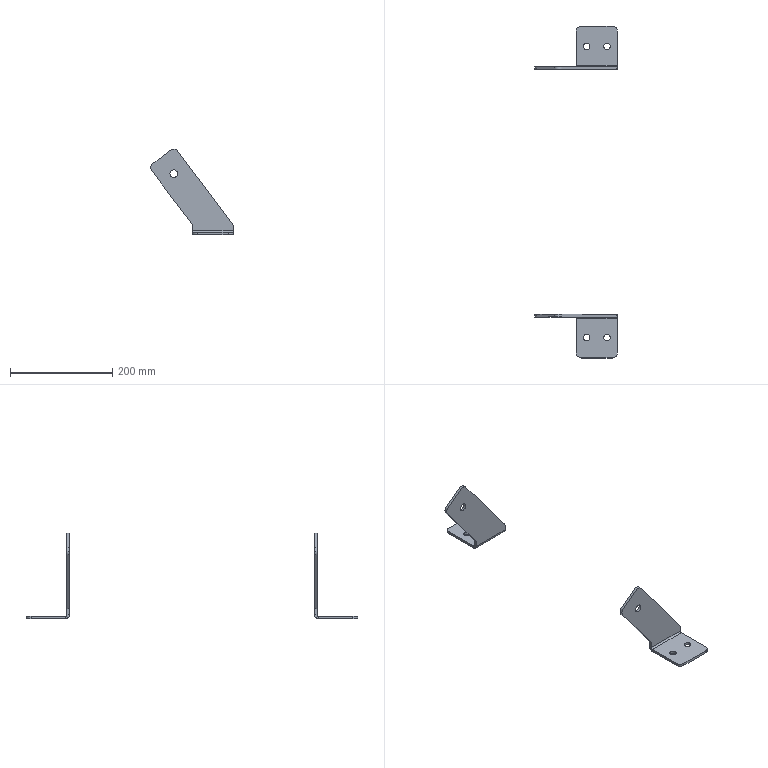Part | STEP file | FEEDER_ANGLESV11 | 2 solids | 56 faces | box 161.429 x 650 x 167.947 mm | volume 179005 mm3 | cylinder 28 | plane 28 | commonest cylinder face diameters 20 x12 13 x8 15 x4 6 x2 16 x2